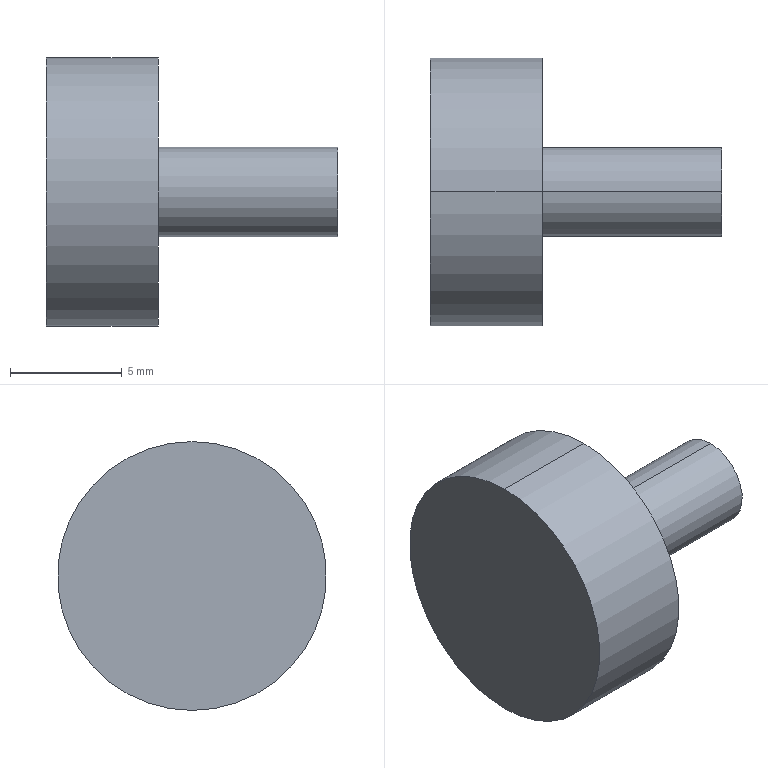Part | SolidWorks | features Revolution 1 | 1 solid | 7 faces | box 13 x 12 x 12 mm | volume 666.018 mm3 | cylinder 4 | plane 3 | commonest cylinder face diameters 4 x2 12 x2
STEP:
#1=CARTESIAN_POINT('',(13.,0.,2.));
#2=VERTEX_POINT('',#1);
#3=CARTESIAN_POINT('',(13.,0.,-2.));
#4=VERTEX_POINT('',#3);
#5=CARTESIAN_POINT('',(13.,0.,0.));
#6=DIRECTION('',(-1.,0.,0.));
#7=DIRECTION('',(0.,0.,1.));
#8=AXIS2_PLACEMENT_3D('',#5,#6,#7);
#9=CIRCLE('',#8,2.);
#10=EDGE_CURVE('',#2,#4,#9,.T.);
#11=ORIENTED_EDGE('',*,*,#10,.T.);
#12=CARTESIAN_POINT('',(5.,0.,-2.));
#13=VERTEX_POINT('',#12);
#14=CARTESIAN_POINT('',(0.,0.,-2.));
#15=DIRECTION('',(-1.,0.,0.));
#16=VECTOR('',#15,1000.);
#17=LINE('',#14,#16);
#18=EDGE_CURVE('',#4,#13,#17,.T.);
#19=ORIENTED_EDGE('',*,*,#18,.T.);
#20=CARTESIAN_POINT('',(5.,0.,2.));
#21=VERTEX_POINT('',#20);
#22=CARTESIAN_POINT('',(5.,0.,0.));
#23=DIRECTION('',(-1.,0.,0.));
#24=DIRECTION('',(0.,0.,1.));
#25=AXIS2_PLACEMENT_3D('',#22,#23,#24);
#26=CIRCLE('',#25,2.);
#27=EDGE_CURVE('',#21,#13,#26,.T.);
#28=ORIENTED_EDGE('',*,*,#27,.F.);
#29=CARTESIAN_POINT('',(0.,0.,2.));
#30=DIRECTION('',(-1.,0.,0.));
#31=VECTOR('',#30,1000.);
#32=LINE('',#29,#31);
#33=EDGE_CURVE('',#2,#21,#32,.T.);
#34=ORIENTED_EDGE('',*,*,#33,.F.);
#35=EDGE_LOOP('',(#11,#19,#28,#34));
#36=FACE_OUTER_BOUND('',#35,.T.);
#37=CARTESIAN_POINT('',(0.,0.,0.));
#38=DIRECTION('',(-1.,0.,0.));
#39=DIRECTION('',(0.,0.,1.));
#40=AXIS2_PLACEMENT_3D('',#37,#38,#39);
#41=CYLINDRICAL_SURFACE('',#40,2.);
#42=ADVANCED_FACE('',(#36),#41,.T.);
#43=CARTESIAN_POINT('',(5.,0.,6.));
#44=VERTEX_POINT('',#43);
#45=CARTESIAN_POINT('',(5.,0.,-6.));
#46=VERTEX_POINT('',#45);
#47=CARTESIAN_POINT('',(5.,0.,0.));
#48=DIRECTION('',(-1.,0.,0.));
#49=DIRECTION('',(0.,0.,1.));
#50=AXIS2_PLACEMENT_3D('',#47,#48,#49);
#51=CIRCLE('',#50,6.);
#52=EDGE_CURVE('',#44,#46,#51,.T.);
#53=ORIENTED_EDGE('',*,*,#52,.T.);
#54=CARTESIAN_POINT('',(0.,0.,-6.));
#55=VERTEX_POINT('',#54);
#56=CARTESIAN_POINT('',(0.,0.,-6.));
#57=DIRECTION('',(-1.,0.,0.));
#58=VECTOR('',#57,1000.);
#59=LINE('',#56,#58);
#60=EDGE_CURVE('',#46,#55,#59,.T.);
#61=ORIENTED_EDGE('',*,*,#60,.T.);
#62=CARTESIAN_POINT('',(0.,0.,6.));
#63=VERTEX_POINT('',#62);
#64=CARTESIAN_POINT('',(0.,0.,0.));
#65=DIRECTION('',(-1.,0.,0.));
#66=DIRECTION('',(0.,0.,1.));
#67=AXIS2_PLACEMENT_3D('',#64,#65,#66);
#68=CIRCLE('',#67,6.);
#69=EDGE_CURVE('',#63,#55,#68,.T.);
#70=ORIENTED_EDGE('',*,*,#69,.F.);
#71=CARTESIAN_POINT('',(0.,0.,6.));
#72=DIRECTION('',(-1.,0.,0.));
#73=VECTOR('',#72,1000.);
#74=LINE('',#71,#73);
#75=EDGE_CURVE('',#44,#63,#74,.T.);
#76=ORIENTED_EDGE('',*,*,#75,.F.);
#77=EDGE_LOOP('',(#53,#61,#70,#76));
#78=FACE_OUTER_BOUND('',#77,.T.);
#79=CARTESIAN_POINT('',(0.,0.,0.));
#80=DIRECTION('',(-1.,0.,0.));
#81=DIRECTION('',(0.,0.,1.));
#82=AXIS2_PLACEMENT_3D('',#79,#80,#81);
#83=CYLINDRICAL_SURFACE('',#82,6.);
#84=ADVANCED_FACE('',(#78),#83,.T.);
#85=ORIENTED_EDGE('',*,*,#69,.T.);
#86=CARTESIAN_POINT('',(0.,0.,0.));
#87=DIRECTION('',(-1.,0.,0.));
#88=DIRECTION('',(0.,0.,1.));
#89=AXIS2_PLACEMENT_3D('',#86,#87,#88);
#90=CIRCLE('',#89,6.);
#91=EDGE_CURVE('',#55,#63,#90,.T.);
#92=ORIENTED_EDGE('',*,*,#91,.T.);
#93=EDGE_LOOP('',(#85,#92));
#94=FACE_OUTER_BOUND('',#93,.T.);
#95=CARTESIAN_POINT('',(0.,0.,0.));
#96=DIRECTION('',(1.,0.,0.));
#97=DIRECTION('',(0.,0.,-1.));
#98=AXIS2_PLACEMENT_3D('',#95,#96,#97);
#99=PLANE('',#98);
#100=ADVANCED_FACE('',(#94),#99,.F.);
#101=ORIENTED_EDGE('',*,*,#60,.F.);
#102=CARTESIAN_POINT('',(5.,0.,0.));
#103=DIRECTION('',(-1.,0.,0.));
#104=DIRECTION('',(0.,0.,1.));
#105=AXIS2_PLACEMENT_3D('',#102,#103,#104);
#106=CIRCLE('',#105,6.);
#107=EDGE_CURVE('',#46,#44,#106,.T.);
#108=ORIENTED_EDGE('',*,*,#107,.T.);
#109=ORIENTED_EDGE('',*,*,#75,.T.);
#110=ORIENTED_EDGE('',*,*,#91,.F.);
#111=EDGE_LOOP('',(#101,#108,#109,#110));
#112=FACE_OUTER_BOUND('',#111,.T.);
#113=CARTESIAN_POINT('',(0.,0.,0.));
#114=DIRECTION('',(-1.,0.,0.));
#115=DIRECTION('',(0.,0.,1.));
#116=AXIS2_PLACEMENT_3D('',#113,#114,#115);
#117=CYLINDRICAL_SURFACE('',#116,6.);
#118=ADVANCED_FACE('',(#112),#117,.T.);
#119=ORIENTED_EDGE('',*,*,#52,.F.);
#120=ORIENTED_EDGE('',*,*,#107,.F.);
#121=EDGE_LOOP('',(#119,#120));
#122=FACE_OUTER_BOUND('',#121,.T.);
#123=ORIENTED_EDGE('',*,*,#27,.T.);
#124=CARTESIAN_POINT('',(5.,0.,0.));
#125=DIRECTION('',(-1.,0.,0.));
#126=DIRECTION('',(0.,0.,1.));
#127=AXIS2_PLACEMENT_3D('',#124,#125,#126);
#128=CIRCLE('',#127,2.);
#129=EDGE_CURVE('',#13,#21,#128,.T.);
#130=ORIENTED_EDGE('',*,*,#129,.T.);
#131=EDGE_LOOP('',(#123,#130));
#132=FACE_BOUND('',#131,.T.);
#133=CARTESIAN_POINT('',(5.,6.,0.));
#134=DIRECTION('',(-1.,0.,0.));
#135=DIRECTION('',(0.,0.,1.));
#136=AXIS2_PLACEMENT_3D('',#133,#134,#135);
#137=PLANE('',#136);
#138=ADVANCED_FACE('',(#122,#132),#137,.F.);
#139=ORIENTED_EDGE('',*,*,#18,.F.);
#140=CARTESIAN_POINT('',(13.,0.,0.));
#141=DIRECTION('',(-1.,0.,0.));
#142=DIRECTION('',(0.,0.,1.));
#143=AXIS2_PLACEMENT_3D('',#140,#141,#142);
#144=CIRCLE('',#143,2.);
#145=EDGE_CURVE('',#4,#2,#144,.T.);
#146=ORIENTED_EDGE('',*,*,#145,.T.);
#147=ORIENTED_EDGE('',*,*,#33,.T.);
#148=ORIENTED_EDGE('',*,*,#129,.F.);
#149=EDGE_LOOP('',(#139,#146,#147,#148));
#150=FACE_OUTER_BOUND('',#149,.T.);
#151=CARTESIAN_POINT('',(0.,0.,0.));
#152=DIRECTION('',(-1.,0.,0.));
#153=DIRECTION('',(0.,0.,1.));
#154=AXIS2_PLACEMENT_3D('',#151,#152,#153);
#155=CYLINDRICAL_SURFACE('',#154,2.);
#156=ADVANCED_FACE('',(#150),#155,.T.);
#157=ORIENTED_EDGE('',*,*,#10,.F.);
#158=ORIENTED_EDGE('',*,*,#145,.F.);
#159=EDGE_LOOP('',(#157,#158));
#160=FACE_OUTER_BOUND('',#159,.T.);
#161=CARTESIAN_POINT('',(13.,2.,0.));
#162=DIRECTION('',(-1.,0.,0.));
#163=DIRECTION('',(0.,0.,1.));
#164=AXIS2_PLACEMENT_3D('',#161,#162,#163);
#165=PLANE('',#164);
#166=ADVANCED_FACE('',(#160),#165,.F.);
#167=CLOSED_SHELL('',(#42,#84,#100,#118,#138,#156,#166));
#168=MANIFOLD_SOLID_BREP('',#167);
#169=CARTESIAN_POINT('',(0.,0.,0.));
#170=DIRECTION('',(0.,0.,1.));
#171=DIRECTION('',(1.,0.,0.));
#172=AXIS2_PLACEMENT_3D('',#169,#170,#171);
#173=(LENGTH_UNIT()NAMED_UNIT(*)SI_UNIT(.MILLI.,.METRE.));
#174=UNCERTAINTY_MEASURE_WITH_UNIT(LENGTH_MEASURE(0.00001),#173,'','');
#175=(NAMED_UNIT(*)PLANE_ANGLE_UNIT()SI_UNIT($,.RADIAN.));
#176=(NAMED_UNIT(*)SI_UNIT($,.STERADIAN.)SOLID_ANGLE_UNIT());
#177=(GEOMETRIC_REPRESENTATION_CONTEXT(3)GLOBAL_UNCERTAINTY_ASSIGNED_CONTEXT((#174))GLOBAL_UNIT_ASSIGNED_CONTEXT((#173,#175,#176))REPRESENTATION_CONTEXT('',''));
#178=ADVANCED_BREP_SHAPE_REPRESENTATION('',(#168,#172),#177);